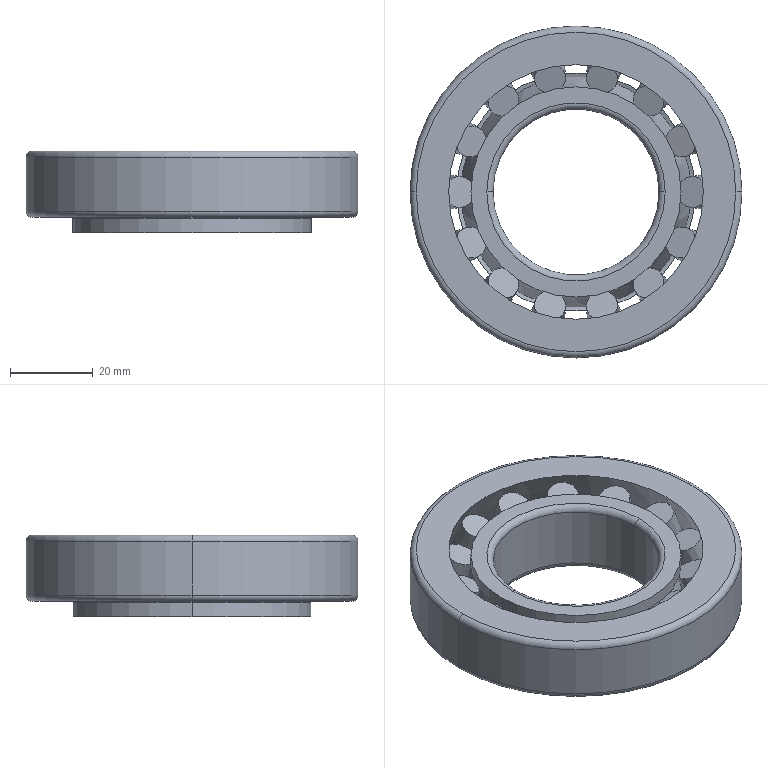Part | SolidWorks | features Revolution 3, CirPattern 1, RefAxis 1 | 16 solids | 84 faces | box 80 x 80 x 19.75 mm | volume 47853 mm3 | cone 36 | plane 32 | torus 8 | cylinder 8 | commonest cylinder face diameters 40 x2 50.653 x2 57.472 x2 80 x2